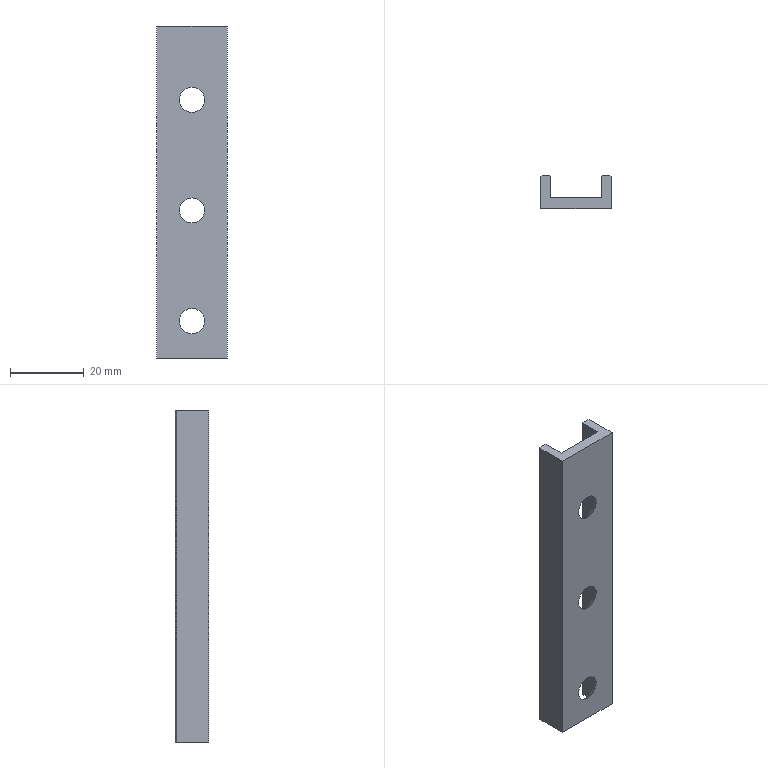Part | SolidWorks | features Chamfer 1, Extrusion 1, HoleWzd 1, LPattern 1 | 1 solid | 20 faces | box 19 x 9 x 90 mm | volume 7114 mm3 | plane 14 | cone 6
STEP:
#1=CARTESIAN_POINT('',(0.,-4.5,66.6));
#2=VERTEX_POINT('',#1);
#3=CARTESIAN_POINT('',(0.,-4.5,73.4));
#4=VERTEX_POINT('',#3);
#5=CARTESIAN_POINT('',(0.,-4.5,70.));
#6=DIRECTION('',(0.,1.,0.));
#7=DIRECTION('',(0.,0.,1.));
#8=AXIS2_PLACEMENT_3D('',#5,#6,#7);
#9=CIRCLE('',#8,3.4);
#10=EDGE_CURVE('',#2,#4,#9,.T.);
#11=ORIENTED_EDGE('',*,*,#10,.F.);
#12=CARTESIAN_POINT('',(0.,-1.5,63.6));
#13=VERTEX_POINT('',#12);
#14=CARTESIAN_POINT('',(0.,-1.5,63.6));
#15=DIRECTION('',(0.,0.7071,-0.7071));
#16=VECTOR('',#15,1000.);
#17=LINE('',#14,#16);
#18=EDGE_CURVE('',#2,#13,#17,.T.);
#19=ORIENTED_EDGE('',*,*,#18,.T.);
#20=CARTESIAN_POINT('',(0.,-1.5,76.4));
#21=VERTEX_POINT('',#20);
#22=CARTESIAN_POINT('',(0.,-1.5,70.));
#23=DIRECTION('',(0.,1.,0.));
#24=DIRECTION('',(0.,0.,1.));
#25=AXIS2_PLACEMENT_3D('',#22,#23,#24);
#26=CIRCLE('',#25,6.4);
#27=EDGE_CURVE('',#13,#21,#26,.T.);
#28=ORIENTED_EDGE('',*,*,#27,.T.);
#29=CARTESIAN_POINT('',(0.,-1.5,76.4));
#30=DIRECTION('',(0.,0.7071,0.7071));
#31=VECTOR('',#30,1000.);
#32=LINE('',#29,#31);
#33=EDGE_CURVE('',#4,#21,#32,.T.);
#34=ORIENTED_EDGE('',*,*,#33,.F.);
#35=EDGE_LOOP('',(#11,#19,#28,#34));
#36=FACE_OUTER_BOUND('',#35,.T.);
#37=CARTESIAN_POINT('',(0.,-1.5,70.));
#38=DIRECTION('',(0.,1.,0.));
#39=DIRECTION('',(0.,0.,1.));
#40=AXIS2_PLACEMENT_3D('',#37,#38,#39);
#41=CONICAL_SURFACE('',#40,6.4,0.7854);
#42=ADVANCED_FACE('',(#36),#41,.F.);
#43=CARTESIAN_POINT('',(0.,-4.5,6.6));
#44=VERTEX_POINT('',#43);
#45=CARTESIAN_POINT('',(0.,-4.5,13.4));
#46=VERTEX_POINT('',#45);
#47=CARTESIAN_POINT('',(0.,-4.5,10.));
#48=DIRECTION('',(0.,1.,0.));
#49=DIRECTION('',(0.,0.,1.));
#50=AXIS2_PLACEMENT_3D('',#47,#48,#49);
#51=CIRCLE('',#50,3.4);
#52=EDGE_CURVE('',#44,#46,#51,.T.);
#53=ORIENTED_EDGE('',*,*,#52,.F.);
#54=CARTESIAN_POINT('',(0.,-1.5,3.6));
#55=VERTEX_POINT('',#54);
#56=CARTESIAN_POINT('',(0.,-1.5,3.6));
#57=DIRECTION('',(0.,0.7071,-0.7071));
#58=VECTOR('',#57,1000.);
#59=LINE('',#56,#58);
#60=EDGE_CURVE('',#44,#55,#59,.T.);
#61=ORIENTED_EDGE('',*,*,#60,.T.);
#62=CARTESIAN_POINT('',(0.,-1.5,16.4));
#63=VERTEX_POINT('',#62);
#64=CARTESIAN_POINT('',(0.,-1.5,10.));
#65=DIRECTION('',(0.,1.,0.));
#66=DIRECTION('',(0.,0.,1.));
#67=AXIS2_PLACEMENT_3D('',#64,#65,#66);
#68=CIRCLE('',#67,6.4);
#69=EDGE_CURVE('',#55,#63,#68,.T.);
#70=ORIENTED_EDGE('',*,*,#69,.T.);
#71=CARTESIAN_POINT('',(0.,-1.5,16.4));
#72=DIRECTION('',(0.,0.7071,0.7071));
#73=VECTOR('',#72,1000.);
#74=LINE('',#71,#73);
#75=EDGE_CURVE('',#46,#63,#74,.T.);
#76=ORIENTED_EDGE('',*,*,#75,.F.);
#77=EDGE_LOOP('',(#53,#61,#70,#76));
#78=FACE_OUTER_BOUND('',#77,.T.);
#79=CARTESIAN_POINT('',(0.,-1.5,10.));
#80=DIRECTION('',(0.,1.,0.));
#81=DIRECTION('',(0.,0.,1.));
#82=AXIS2_PLACEMENT_3D('',#79,#80,#81);
#83=CONICAL_SURFACE('',#82,6.4,0.7854);
#84=ADVANCED_FACE('',(#78),#83,.F.);
#85=CARTESIAN_POINT('',(0.,-4.5,36.6));
#86=VERTEX_POINT('',#85);
#87=CARTESIAN_POINT('',(0.,-4.5,43.4));
#88=VERTEX_POINT('',#87);
#89=CARTESIAN_POINT('',(0.,-4.5,40.));
#90=DIRECTION('',(0.,1.,0.));
#91=DIRECTION('',(0.,0.,1.));
#92=AXIS2_PLACEMENT_3D('',#89,#90,#91);
#93=CIRCLE('',#92,3.4);
#94=EDGE_CURVE('',#86,#88,#93,.T.);
#95=ORIENTED_EDGE('',*,*,#94,.F.);
#96=CARTESIAN_POINT('',(0.,-1.5,33.6));
#97=VERTEX_POINT('',#96);
#98=CARTESIAN_POINT('',(0.,-1.5,33.6));
#99=DIRECTION('',(0.,0.7071,-0.7071));
#100=VECTOR('',#99,1000.);
#101=LINE('',#98,#100);
#102=EDGE_CURVE('',#86,#97,#101,.T.);
#103=ORIENTED_EDGE('',*,*,#102,.T.);
#104=CARTESIAN_POINT('',(0.,-1.5,46.4));
#105=VERTEX_POINT('',#104);
#106=CARTESIAN_POINT('',(0.,-1.5,40.));
#107=DIRECTION('',(0.,1.,0.));
#108=DIRECTION('',(0.,0.,1.));
#109=AXIS2_PLACEMENT_3D('',#106,#107,#108);
#110=CIRCLE('',#109,6.4);
#111=EDGE_CURVE('',#97,#105,#110,.T.);
#112=ORIENTED_EDGE('',*,*,#111,.T.);
#113=CARTESIAN_POINT('',(0.,-1.5,46.4));
#114=DIRECTION('',(0.,0.7071,0.7071));
#115=VECTOR('',#114,1000.);
#116=LINE('',#113,#115);
#117=EDGE_CURVE('',#88,#105,#116,.T.);
#118=ORIENTED_EDGE('',*,*,#117,.F.);
#119=EDGE_LOOP('',(#95,#103,#112,#118));
#120=FACE_OUTER_BOUND('',#119,.T.);
#121=CARTESIAN_POINT('',(0.,-1.5,40.));
#122=DIRECTION('',(0.,1.,0.));
#123=DIRECTION('',(0.,0.,1.));
#124=AXIS2_PLACEMENT_3D('',#121,#122,#123);
#125=CONICAL_SURFACE('',#124,6.4,0.7854);
#126=ADVANCED_FACE('',(#120),#125,.F.);
#127=CARTESIAN_POINT('',(0.,-4.5,70.));
#128=DIRECTION('',(0.,1.,0.));
#129=DIRECTION('',(0.,0.,1.));
#130=AXIS2_PLACEMENT_3D('',#127,#128,#129);
#131=CIRCLE('',#130,3.4);
#132=EDGE_CURVE('',#4,#2,#131,.T.);
#133=ORIENTED_EDGE('',*,*,#132,.T.);
#134=ORIENTED_EDGE('',*,*,#10,.T.);
#135=EDGE_LOOP('',(#133,#134));
#136=FACE_BOUND('',#135,.T.);
#137=CARTESIAN_POINT('',(0.,-4.5,10.));
#138=DIRECTION('',(0.,1.,0.));
#139=DIRECTION('',(0.,0.,1.));
#140=AXIS2_PLACEMENT_3D('',#137,#138,#139);
#141=CIRCLE('',#140,3.4);
#142=EDGE_CURVE('',#46,#44,#141,.T.);
#143=ORIENTED_EDGE('',*,*,#142,.T.);
#144=ORIENTED_EDGE('',*,*,#52,.T.);
#145=EDGE_LOOP('',(#143,#144));
#146=FACE_BOUND('',#145,.T.);
#147=CARTESIAN_POINT('',(0.,-4.5,40.));
#148=DIRECTION('',(0.,1.,0.));
#149=DIRECTION('',(0.,0.,1.));
#150=AXIS2_PLACEMENT_3D('',#147,#148,#149);
#151=CIRCLE('',#150,3.4);
#152=EDGE_CURVE('',#88,#86,#151,.T.);
#153=ORIENTED_EDGE('',*,*,#152,.T.);
#154=ORIENTED_EDGE('',*,*,#94,.T.);
#155=EDGE_LOOP('',(#153,#154));
#156=FACE_BOUND('',#155,.T.);
#157=CARTESIAN_POINT('',(-9.5,-4.5,0.));
#158=VERTEX_POINT('',#157);
#159=CARTESIAN_POINT('',(9.5,-4.5,0.));
#160=VERTEX_POINT('',#159);
#161=CARTESIAN_POINT('',(-9.5,-4.5,0.));
#162=DIRECTION('',(1.,0.,0.));
#163=VECTOR('',#162,1000.);
#164=LINE('',#161,#163);
#165=EDGE_CURVE('',#158,#160,#164,.T.);
#166=ORIENTED_EDGE('',*,*,#165,.T.);
#167=CARTESIAN_POINT('',(9.5,-4.5,90.));
#168=VERTEX_POINT('',#167);
#169=CARTESIAN_POINT('',(9.5,-4.5,90.));
#170=DIRECTION('',(0.,0.,-1.));
#171=VECTOR('',#170,1000.);
#172=LINE('',#169,#171);
#173=EDGE_CURVE('',#168,#160,#172,.T.);
#174=ORIENTED_EDGE('',*,*,#173,.F.);
#175=CARTESIAN_POINT('',(-9.5,-4.5,90.));
#176=VERTEX_POINT('',#175);
#177=CARTESIAN_POINT('',(-9.5,-4.5,90.));
#178=DIRECTION('',(1.,0.,0.));
#179=VECTOR('',#178,1000.);
#180=LINE('',#177,#179);
#181=EDGE_CURVE('',#176,#168,#180,.T.);
#182=ORIENTED_EDGE('',*,*,#181,.F.);
#183=CARTESIAN_POINT('',(-9.5,-4.5,90.));
#184=DIRECTION('',(0.,0.,-1.));
#185=VECTOR('',#184,1000.);
#186=LINE('',#183,#185);
#187=EDGE_CURVE('',#176,#158,#186,.T.);
#188=ORIENTED_EDGE('',*,*,#187,.T.);
#189=EDGE_LOOP('',(#166,#174,#182,#188));
#190=FACE_OUTER_BOUND('',#189,.T.);
#191=CARTESIAN_POINT('',(-9.5,-4.5,90.));
#192=DIRECTION('',(0.,1.,0.));
#193=DIRECTION('',(0.,0.,1.));
#194=AXIS2_PLACEMENT_3D('',#191,#192,#193);
#195=PLANE('',#194);
#196=ADVANCED_FACE('',(#136,#146,#156,#190),#195,.F.);
#197=CARTESIAN_POINT('',(9.2,4.5,90.));
#198=VERTEX_POINT('',#197);
#199=CARTESIAN_POINT('',(7.3,4.5,90.));
#200=VERTEX_POINT('',#199);
#201=CARTESIAN_POINT('',(7.,4.5,90.));
#202=DIRECTION('',(-1.,0.,0.));
#203=VECTOR('',#202,1000.);
#204=LINE('',#201,#203);
#205=EDGE_CURVE('',#198,#200,#204,.T.);
#206=ORIENTED_EDGE('',*,*,#205,.F.);
#207=CARTESIAN_POINT('',(9.2,4.5,0.));
#208=VERTEX_POINT('',#207);
#209=CARTESIAN_POINT('',(9.2,4.5,90.));
#210=DIRECTION('',(0.,0.,-1.));
#211=VECTOR('',#210,1000.);
#212=LINE('',#209,#211);
#213=EDGE_CURVE('',#198,#208,#212,.T.);
#214=ORIENTED_EDGE('',*,*,#213,.T.);
#215=CARTESIAN_POINT('',(7.3,4.5,0.));
#216=VERTEX_POINT('',#215);
#217=CARTESIAN_POINT('',(7.,4.5,0.));
#218=DIRECTION('',(-1.,0.,0.));
#219=VECTOR('',#218,1000.);
#220=LINE('',#217,#219);
#221=EDGE_CURVE('',#208,#216,#220,.T.);
#222=ORIENTED_EDGE('',*,*,#221,.T.);
#223=CARTESIAN_POINT('',(7.3,4.5,90.));
#224=DIRECTION('',(0.,0.,1.));
#225=VECTOR('',#224,1000.);
#226=LINE('',#223,#225);
#227=EDGE_CURVE('',#216,#200,#226,.T.);
#228=ORIENTED_EDGE('',*,*,#227,.T.);
#229=EDGE_LOOP('',(#206,#214,#222,#228));
#230=FACE_OUTER_BOUND('',#229,.T.);
#231=CARTESIAN_POINT('',(7.,4.5,90.));
#232=DIRECTION('',(0.,-1.,0.));
#233=DIRECTION('',(1.,0.,0.));
#234=AXIS2_PLACEMENT_3D('',#231,#232,#233);
#235=PLANE('',#234);
#236=ADVANCED_FACE('',(#230),#235,.F.);
#237=CARTESIAN_POINT('',(7.,4.2,90.));
#238=VERTEX_POINT('',#237);
#239=CARTESIAN_POINT('',(7.,-1.5,90.));
#240=VERTEX_POINT('',#239);
#241=CARTESIAN_POINT('',(7.,-1.5,90.));
#242=DIRECTION('',(0.,-1.,0.));
#243=VECTOR('',#242,1000.);
#244=LINE('',#241,#243);
#245=EDGE_CURVE('',#238,#240,#244,.T.);
#246=ORIENTED_EDGE('',*,*,#245,.F.);
#247=CARTESIAN_POINT('',(7.,4.2,0.));
#248=VERTEX_POINT('',#247);
#249=CARTESIAN_POINT('',(7.,4.2,90.));
#250=DIRECTION('',(0.,0.,-1.));
#251=VECTOR('',#250,1000.);
#252=LINE('',#249,#251);
#253=EDGE_CURVE('',#238,#248,#252,.T.);
#254=ORIENTED_EDGE('',*,*,#253,.T.);
#255=CARTESIAN_POINT('',(7.,-1.5,0.));
#256=VERTEX_POINT('',#255);
#257=CARTESIAN_POINT('',(7.,-1.5,0.));
#258=DIRECTION('',(0.,-1.,0.));
#259=VECTOR('',#258,1000.);
#260=LINE('',#257,#259);
#261=EDGE_CURVE('',#248,#256,#260,.T.);
#262=ORIENTED_EDGE('',*,*,#261,.T.);
#263=CARTESIAN_POINT('',(7.,-1.5,90.));
#264=DIRECTION('',(0.,0.,-1.));
#265=VECTOR('',#264,1000.);
#266=LINE('',#263,#265);
#267=EDGE_CURVE('',#240,#256,#266,.T.);
#268=ORIENTED_EDGE('',*,*,#267,.F.);
#269=EDGE_LOOP('',(#246,#254,#262,#268));
#270=FACE_OUTER_BOUND('',#269,.T.);
#271=CARTESIAN_POINT('',(7.,-1.5,90.));
#272=DIRECTION('',(1.,0.,0.));
#273=DIRECTION('',(0.,1.,0.));
#274=AXIS2_PLACEMENT_3D('',#271,#272,#273);
#275=PLANE('',#274);
#276=ADVANCED_FACE('',(#270),#275,.F.);
#277=CARTESIAN_POINT('',(0.,-1.5,70.));
#278=DIRECTION('',(0.,1.,0.));
#279=DIRECTION('',(0.,0.,1.));
#280=AXIS2_PLACEMENT_3D('',#277,#278,#279);
#281=CIRCLE('',#280,6.4);
#282=EDGE_CURVE('',#21,#13,#281,.T.);
#283=ORIENTED_EDGE('',*,*,#282,.F.);
#284=ORIENTED_EDGE('',*,*,#27,.F.);
#285=EDGE_LOOP('',(#283,#284));
#286=FACE_BOUND('',#285,.T.);
#287=CARTESIAN_POINT('',(0.,-1.5,10.));
#288=DIRECTION('',(0.,1.,0.));
#289=DIRECTION('',(0.,0.,1.));
#290=AXIS2_PLACEMENT_3D('',#287,#288,#289);
#291=CIRCLE('',#290,6.4);
#292=EDGE_CURVE('',#63,#55,#291,.T.);
#293=ORIENTED_EDGE('',*,*,#292,.F.);
#294=ORIENTED_EDGE('',*,*,#69,.F.);
#295=EDGE_LOOP('',(#293,#294));
#296=FACE_BOUND('',#295,.T.);
#297=CARTESIAN_POINT('',(0.,-1.5,40.));
#298=DIRECTION('',(0.,1.,0.));
#299=DIRECTION('',(0.,0.,1.));
#300=AXIS2_PLACEMENT_3D('',#297,#298,#299);
#301=CIRCLE('',#300,6.4);
#302=EDGE_CURVE('',#105,#97,#301,.T.);
#303=ORIENTED_EDGE('',*,*,#302,.F.);
#304=ORIENTED_EDGE('',*,*,#111,.F.);
#305=EDGE_LOOP('',(#303,#304));
#306=FACE_BOUND('',#305,.T.);
#307=CARTESIAN_POINT('',(-7.,-1.5,0.));
#308=VERTEX_POINT('',#307);
#309=CARTESIAN_POINT('',(-7.,-1.5,0.));
#310=DIRECTION('',(-1.,0.,0.));
#311=VECTOR('',#310,1000.);
#312=LINE('',#309,#311);
#313=EDGE_CURVE('',#256,#308,#312,.T.);
#314=ORIENTED_EDGE('',*,*,#313,.T.);
#315=CARTESIAN_POINT('',(-7.,-1.5,90.));
#316=VERTEX_POINT('',#315);
#317=CARTESIAN_POINT('',(-7.,-1.5,90.));
#318=DIRECTION('',(0.,0.,-1.));
#319=VECTOR('',#318,1000.);
#320=LINE('',#317,#319);
#321=EDGE_CURVE('',#316,#308,#320,.T.);
#322=ORIENTED_EDGE('',*,*,#321,.F.);
#323=CARTESIAN_POINT('',(-7.,-1.5,90.));
#324=DIRECTION('',(-1.,0.,0.));
#325=VECTOR('',#324,1000.);
#326=LINE('',#323,#325);
#327=EDGE_CURVE('',#240,#316,#326,.T.);
#328=ORIENTED_EDGE('',*,*,#327,.F.);
#329=ORIENTED_EDGE('',*,*,#267,.T.);
#330=EDGE_LOOP('',(#314,#322,#328,#329));
#331=FACE_OUTER_BOUND('',#330,.T.);
#332=CARTESIAN_POINT('',(-7.,-1.5,90.));
#333=DIRECTION('',(0.,-1.,0.));
#334=DIRECTION('',(1.,0.,0.));
#335=AXIS2_PLACEMENT_3D('',#332,#333,#334);
#336=PLANE('',#335);
#337=ADVANCED_FACE('',(#286,#296,#306,#331),#336,.F.);
#338=CARTESIAN_POINT('',(-7.,4.2,0.));
#339=VERTEX_POINT('',#338);
#340=CARTESIAN_POINT('',(-7.,4.5,0.));
#341=DIRECTION('',(0.,1.,0.));
#342=VECTOR('',#341,1000.);
#343=LINE('',#340,#342);
#344=EDGE_CURVE('',#308,#339,#343,.T.);
#345=ORIENTED_EDGE('',*,*,#344,.T.);
#346=CARTESIAN_POINT('',(-7.,4.2,90.));
#347=VERTEX_POINT('',#346);
#348=CARTESIAN_POINT('',(-7.,4.2,90.));
#349=DIRECTION('',(0.,0.,1.));
#350=VECTOR('',#349,1000.);
#351=LINE('',#348,#350);
#352=EDGE_CURVE('',#339,#347,#351,.T.);
#353=ORIENTED_EDGE('',*,*,#352,.T.);
#354=CARTESIAN_POINT('',(-7.,4.5,90.));
#355=DIRECTION('',(0.,1.,0.));
#356=VECTOR('',#355,1000.);
#357=LINE('',#354,#356);
#358=EDGE_CURVE('',#316,#347,#357,.T.);
#359=ORIENTED_EDGE('',*,*,#358,.F.);
#360=ORIENTED_EDGE('',*,*,#321,.T.);
#361=EDGE_LOOP('',(#345,#353,#359,#360));
#362=FACE_OUTER_BOUND('',#361,.T.);
#363=CARTESIAN_POINT('',(-7.,4.5,90.));
#364=DIRECTION('',(-1.,0.,0.));
#365=DIRECTION('',(0.,-1.,0.));
#366=AXIS2_PLACEMENT_3D('',#363,#364,#365);
#367=PLANE('',#366);
#368=ADVANCED_FACE('',(#362),#367,.F.);
#369=CARTESIAN_POINT('',(-7.3,4.5,0.));
#370=VERTEX_POINT('',#369);
#371=CARTESIAN_POINT('',(-9.2,4.5,0.));
#372=VERTEX_POINT('',#371);
#373=CARTESIAN_POINT('',(-9.5,4.5,0.));
#374=DIRECTION('',(-1.,0.,0.));
#375=VECTOR('',#374,1000.);
#376=LINE('',#373,#375);
#377=EDGE_CURVE('',#370,#372,#376,.T.);
#378=ORIENTED_EDGE('',*,*,#377,.T.);
#379=CARTESIAN_POINT('',(-9.2,4.5,90.));
#380=VERTEX_POINT('',#379);
#381=CARTESIAN_POINT('',(-9.2,4.5,90.));
#382=DIRECTION('',(0.,0.,1.));
#383=VECTOR('',#382,1000.);
#384=LINE('',#381,#383);
#385=EDGE_CURVE('',#372,#380,#384,.T.);
#386=ORIENTED_EDGE('',*,*,#385,.T.);
#387=CARTESIAN_POINT('',(-7.3,4.5,90.));
#388=VERTEX_POINT('',#387);
#389=CARTESIAN_POINT('',(-9.5,4.5,90.));
#390=DIRECTION('',(-1.,0.,0.));
#391=VECTOR('',#390,1000.);
#392=LINE('',#389,#391);
#393=EDGE_CURVE('',#388,#380,#392,.T.);
#394=ORIENTED_EDGE('',*,*,#393,.F.);
#395=CARTESIAN_POINT('',(-7.3,4.5,90.));
#396=DIRECTION('',(0.,0.,-1.));
#397=VECTOR('',#396,1000.);
#398=LINE('',#395,#397);
#399=EDGE_CURVE('',#388,#370,#398,.T.);
#400=ORIENTED_EDGE('',*,*,#399,.T.);
#401=EDGE_LOOP('',(#378,#386,#394,#400));
#402=FACE_OUTER_BOUND('',#401,.T.);
#403=CARTESIAN_POINT('',(-9.5,4.5,90.));
#404=DIRECTION('',(0.,-1.,0.));
#405=DIRECTION('',(1.,0.,0.));
#406=AXIS2_PLACEMENT_3D('',#403,#404,#405);
#407=PLANE('',#406);
#408=ADVANCED_FACE('',(#402),#407,.F.);
#409=CARTESIAN_POINT('',(-9.5,4.2,90.));
#410=VERTEX_POINT('',#409);
#411=CARTESIAN_POINT('',(-9.5,-4.5,90.));
#412=DIRECTION('',(0.,-1.,0.));
#413=VECTOR('',#412,1000.);
#414=LINE('',#411,#413);
#415=EDGE_CURVE('',#410,#176,#414,.T.);
#416=ORIENTED_EDGE('',*,*,#415,.F.);
#417=CARTESIAN_POINT('',(-9.5,4.2,0.));
#418=VERTEX_POINT('',#417);
#419=CARTESIAN_POINT('',(-9.5,4.2,90.));
#420=DIRECTION('',(0.,0.,-1.));
#421=VECTOR('',#420,1000.);
#422=LINE('',#419,#421);
#423=EDGE_CURVE('',#410,#418,#422,.T.);
#424=ORIENTED_EDGE('',*,*,#423,.T.);
#425=CARTESIAN_POINT('',(-9.5,-4.5,0.));
#426=DIRECTION('',(0.,-1.,0.));
#427=VECTOR('',#426,1000.);
#428=LINE('',#425,#427);
#429=EDGE_CURVE('',#418,#158,#428,.T.);
#430=ORIENTED_EDGE('',*,*,#429,.T.);
#431=ORIENTED_EDGE('',*,*,#187,.F.);
#432=EDGE_LOOP('',(#416,#424,#430,#431));
#433=FACE_OUTER_BOUND('',#432,.T.);
#434=CARTESIAN_POINT('',(-9.5,-4.5,90.));
#435=DIRECTION('',(1.,0.,0.));
#436=DIRECTION('',(0.,0.,-1.));
#437=AXIS2_PLACEMENT_3D('',#434,#435,#436);
#438=PLANE('',#437);
#439=ADVANCED_FACE('',(#433),#438,.F.);
#440=CARTESIAN_POINT('',(9.5,4.2,0.));
#441=VERTEX_POINT('',#440);
#442=CARTESIAN_POINT('',(9.5,-4.5,0.));
#443=DIRECTION('',(0.,1.,0.));
#444=VECTOR('',#443,1000.);
#445=LINE('',#442,#444);
#446=EDGE_CURVE('',#160,#441,#445,.T.);
#447=ORIENTED_EDGE('',*,*,#446,.T.);
#448=CARTESIAN_POINT('',(9.5,4.2,90.));
#449=VERTEX_POINT('',#448);
#450=CARTESIAN_POINT('',(9.5,4.2,90.));
#451=DIRECTION('',(0.,0.,1.));
#452=VECTOR('',#451,1000.);
#453=LINE('',#450,#452);
#454=EDGE_CURVE('',#441,#449,#453,.T.);
#455=ORIENTED_EDGE('',*,*,#454,.T.);
#456=CARTESIAN_POINT('',(9.5,-4.5,90.));
#457=DIRECTION('',(0.,1.,0.));
#458=VECTOR('',#457,1000.);
#459=LINE('',#456,#458);
#460=EDGE_CURVE('',#168,#449,#459,.T.);
#461=ORIENTED_EDGE('',*,*,#460,.F.);
#462=ORIENTED_EDGE('',*,*,#173,.T.);
#463=EDGE_LOOP('',(#447,#455,#461,#462));
#464=FACE_OUTER_BOUND('',#463,.T.);
#465=CARTESIAN_POINT('',(9.5,-4.5,90.));
#466=DIRECTION('',(-1.,0.,0.));
#467=DIRECTION('',(0.,0.,1.));
#468=AXIS2_PLACEMENT_3D('',#465,#466,#467);
#469=PLANE('',#468);
#470=ADVANCED_FACE('',(#464),#469,.F.);
#471=ORIENTED_EDGE('',*,*,#393,.T.);
#472=CARTESIAN_POINT('',(-6.85,6.85,90.));
#473=DIRECTION('',(-0.7071,-0.7071,0.));
#474=VECTOR('',#473,1000.);
#475=LINE('',#472,#474);
#476=EDGE_CURVE('',#380,#410,#475,.T.);
#477=ORIENTED_EDGE('',*,*,#476,.T.);
#478=ORIENTED_EDGE('',*,*,#415,.T.);
#479=ORIENTED_EDGE('',*,*,#181,.T.);
#480=ORIENTED_EDGE('',*,*,#460,.T.);
#481=CARTESIAN_POINT('',(6.85,6.85,90.));
#482=DIRECTION('',(-0.7071,0.7071,0.));
#483=VECTOR('',#482,1000.);
#484=LINE('',#481,#483);
#485=EDGE_CURVE('',#449,#198,#484,.T.);
#486=ORIENTED_EDGE('',*,*,#485,.T.);
#487=ORIENTED_EDGE('',*,*,#205,.T.);
#488=CARTESIAN_POINT('',(1.4,-1.4,90.));
#489=DIRECTION('',(-0.7071,-0.7071,0.));
#490=VECTOR('',#489,1000.);
#491=LINE('',#488,#490);
#492=EDGE_CURVE('',#200,#238,#491,.T.);
#493=ORIENTED_EDGE('',*,*,#492,.T.);
#494=ORIENTED_EDGE('',*,*,#245,.T.);
#495=ORIENTED_EDGE('',*,*,#327,.T.);
#496=ORIENTED_EDGE('',*,*,#358,.T.);
#497=CARTESIAN_POINT('',(-1.4,-1.4,90.));
#498=DIRECTION('',(-0.7071,0.7071,0.));
#499=VECTOR('',#498,1000.);
#500=LINE('',#497,#499);
#501=EDGE_CURVE('',#347,#388,#500,.T.);
#502=ORIENTED_EDGE('',*,*,#501,.T.);
#503=EDGE_LOOP('',(#471,#477,#478,#479,#480,#486,#487,#493,#494,#495,#496,#502));
#504=FACE_OUTER_BOUND('',#503,.T.);
#505=CARTESIAN_POINT('',(0.,0.,90.));
#506=DIRECTION('',(0.,0.,1.));
#507=DIRECTION('',(1.,0.,0.));
#508=AXIS2_PLACEMENT_3D('',#505,#506,#507);
#509=PLANE('',#508);
#510=ADVANCED_FACE('',(#504),#509,.T.);
#511=ORIENTED_EDGE('',*,*,#429,.F.);
#512=CARTESIAN_POINT('',(-9.5,4.2,0.));
#513=DIRECTION('',(0.7071,0.7071,0.));
#514=VECTOR('',#513,1000.);
#515=LINE('',#512,#514);
#516=EDGE_CURVE('',#418,#372,#515,.T.);
#517=ORIENTED_EDGE('',*,*,#516,.T.);
#518=ORIENTED_EDGE('',*,*,#377,.F.);
#519=CARTESIAN_POINT('',(-7.3,4.5,0.));
#520=DIRECTION('',(0.7071,-0.7071,0.));
#521=VECTOR('',#520,1000.);
#522=LINE('',#519,#521);
#523=EDGE_CURVE('',#370,#339,#522,.T.);
#524=ORIENTED_EDGE('',*,*,#523,.T.);
#525=ORIENTED_EDGE('',*,*,#344,.F.);
#526=ORIENTED_EDGE('',*,*,#313,.F.);
#527=ORIENTED_EDGE('',*,*,#261,.F.);
#528=CARTESIAN_POINT('',(7.,4.2,0.));
#529=DIRECTION('',(0.7071,0.7071,0.));
#530=VECTOR('',#529,1000.);
#531=LINE('',#528,#530);
#532=EDGE_CURVE('',#248,#216,#531,.T.);
#533=ORIENTED_EDGE('',*,*,#532,.T.);
#534=ORIENTED_EDGE('',*,*,#221,.F.);
#535=CARTESIAN_POINT('',(9.2,4.5,0.));
#536=DIRECTION('',(0.7071,-0.7071,0.));
#537=VECTOR('',#536,1000.);
#538=LINE('',#535,#537);
#539=EDGE_CURVE('',#208,#441,#538,.T.);
#540=ORIENTED_EDGE('',*,*,#539,.T.);
#541=ORIENTED_EDGE('',*,*,#446,.F.);
#542=ORIENTED_EDGE('',*,*,#165,.F.);
#543=EDGE_LOOP('',(#511,#517,#518,#524,#525,#526,#527,#533,#534,#540,#541,#542));
#544=FACE_OUTER_BOUND('',#543,.T.);
#545=CARTESIAN_POINT('',(0.,0.,0.));
#546=DIRECTION('',(0.,0.,1.));
#547=DIRECTION('',(1.,0.,0.));
#548=AXIS2_PLACEMENT_3D('',#545,#546,#547);
#549=PLANE('',#548);
#550=ADVANCED_FACE('',(#544),#549,.F.);
#551=ORIENTED_EDGE('',*,*,#102,.F.);
#552=ORIENTED_EDGE('',*,*,#152,.F.);
#553=ORIENTED_EDGE('',*,*,#117,.T.);
#554=ORIENTED_EDGE('',*,*,#302,.T.);
#555=EDGE_LOOP('',(#551,#552,#553,#554));
#556=FACE_OUTER_BOUND('',#555,.T.);
#557=CARTESIAN_POINT('',(0.,-1.5,40.));
#558=DIRECTION('',(0.,1.,0.));
#559=DIRECTION('',(0.,0.,1.));
#560=AXIS2_PLACEMENT_3D('',#557,#558,#559);
#561=CONICAL_SURFACE('',#560,6.4,0.7854);
#562=ADVANCED_FACE('',(#556),#561,.F.);
#563=ORIENTED_EDGE('',*,*,#60,.F.);
#564=ORIENTED_EDGE('',*,*,#142,.F.);
#565=ORIENTED_EDGE('',*,*,#75,.T.);
#566=ORIENTED_EDGE('',*,*,#292,.T.);
#567=EDGE_LOOP('',(#563,#564,#565,#566));
#568=FACE_OUTER_BOUND('',#567,.T.);
#569=CARTESIAN_POINT('',(0.,-1.5,10.));
#570=DIRECTION('',(0.,1.,0.));
#571=DIRECTION('',(0.,0.,1.));
#572=AXIS2_PLACEMENT_3D('',#569,#570,#571);
#573=CONICAL_SURFACE('',#572,6.4,0.7854);
#574=ADVANCED_FACE('',(#568),#573,.F.);
#575=ORIENTED_EDGE('',*,*,#18,.F.);
#576=ORIENTED_EDGE('',*,*,#132,.F.);
#577=ORIENTED_EDGE('',*,*,#33,.T.);
#578=ORIENTED_EDGE('',*,*,#282,.T.);
#579=EDGE_LOOP('',(#575,#576,#577,#578));
#580=FACE_OUTER_BOUND('',#579,.T.);
#581=CARTESIAN_POINT('',(0.,-1.5,70.));
#582=DIRECTION('',(0.,1.,0.));
#583=DIRECTION('',(0.,0.,1.));
#584=AXIS2_PLACEMENT_3D('',#581,#582,#583);
#585=CONICAL_SURFACE('',#584,6.4,0.7854);
#586=ADVANCED_FACE('',(#580),#585,.F.);
#587=ORIENTED_EDGE('',*,*,#476,.F.);
#588=ORIENTED_EDGE('',*,*,#385,.F.);
#589=ORIENTED_EDGE('',*,*,#516,.F.);
#590=ORIENTED_EDGE('',*,*,#423,.F.);
#591=EDGE_LOOP('',(#587,#588,#589,#590));
#592=FACE_OUTER_BOUND('',#591,.T.);
#593=CARTESIAN_POINT('',(-9.5,4.2,90.));
#594=DIRECTION('',(0.7071,-0.7071,0.));
#595=DIRECTION('',(0.,0.,-1.));
#596=AXIS2_PLACEMENT_3D('',#593,#594,#595);
#597=PLANE('',#596);
#598=ADVANCED_FACE('',(#592),#597,.F.);
#599=ORIENTED_EDGE('',*,*,#485,.F.);
#600=ORIENTED_EDGE('',*,*,#454,.F.);
#601=ORIENTED_EDGE('',*,*,#539,.F.);
#602=ORIENTED_EDGE('',*,*,#213,.F.);
#603=EDGE_LOOP('',(#599,#600,#601,#602));
#604=FACE_OUTER_BOUND('',#603,.T.);
#605=CARTESIAN_POINT('',(9.2,4.5,90.));
#606=DIRECTION('',(-0.7071,-0.7071,0.));
#607=DIRECTION('',(0.,0.,-1.));
#608=AXIS2_PLACEMENT_3D('',#605,#606,#607);
#609=PLANE('',#608);
#610=ADVANCED_FACE('',(#604),#609,.F.);
#611=ORIENTED_EDGE('',*,*,#501,.F.);
#612=ORIENTED_EDGE('',*,*,#352,.F.);
#613=ORIENTED_EDGE('',*,*,#523,.F.);
#614=ORIENTED_EDGE('',*,*,#399,.F.);
#615=EDGE_LOOP('',(#611,#612,#613,#614));
#616=FACE_OUTER_BOUND('',#615,.T.);
#617=CARTESIAN_POINT('',(-7.3,4.5,90.));
#618=DIRECTION('',(-0.7071,-0.7071,0.));
#619=DIRECTION('',(0.,0.,-1.));
#620=AXIS2_PLACEMENT_3D('',#617,#618,#619);
#621=PLANE('',#620);
#622=ADVANCED_FACE('',(#616),#621,.F.);
#623=ORIENTED_EDGE('',*,*,#492,.F.);
#624=ORIENTED_EDGE('',*,*,#227,.F.);
#625=ORIENTED_EDGE('',*,*,#532,.F.);
#626=ORIENTED_EDGE('',*,*,#253,.F.);
#627=EDGE_LOOP('',(#623,#624,#625,#626));
#628=FACE_OUTER_BOUND('',#627,.T.);
#629=CARTESIAN_POINT('',(7.,4.2,90.));
#630=DIRECTION('',(0.7071,-0.7071,0.));
#631=DIRECTION('',(0.,0.,-1.));
#632=AXIS2_PLACEMENT_3D('',#629,#630,#631);
#633=PLANE('',#632);
#634=ADVANCED_FACE('',(#628),#633,.F.);
#635=CLOSED_SHELL('',(#42,#84,#126,#196,#236,#276,#337,#368,#408,#439,#470,#510,#550,#562,#574,#586,#598,#610,#622,#634));
#636=MANIFOLD_SOLID_BREP('',#635);
#637=CARTESIAN_POINT('',(0.,0.,0.));
#638=DIRECTION('',(0.,0.,1.));
#639=DIRECTION('',(1.,0.,0.));
#640=AXIS2_PLACEMENT_3D('',#637,#638,#639);
#641=(LENGTH_UNIT()NAMED_UNIT(*)SI_UNIT(.MILLI.,.METRE.));
#642=UNCERTAINTY_MEASURE_WITH_UNIT(LENGTH_MEASURE(0.00001),#641,'','');
#643=(NAMED_UNIT(*)PLANE_ANGLE_UNIT()SI_UNIT($,.RADIAN.));
#644=(NAMED_UNIT(*)SI_UNIT($,.STERADIAN.)SOLID_ANGLE_UNIT());
#645=(GEOMETRIC_REPRESENTATION_CONTEXT(3)GLOBAL_UNCERTAINTY_ASSIGNED_CONTEXT((#642))GLOBAL_UNIT_ASSIGNED_CONTEXT((#641,#643,#644))REPRESENTATION_CONTEXT('',''));
#646=ADVANCED_BREP_SHAPE_REPRESENTATION('',(#636,#640),#645);